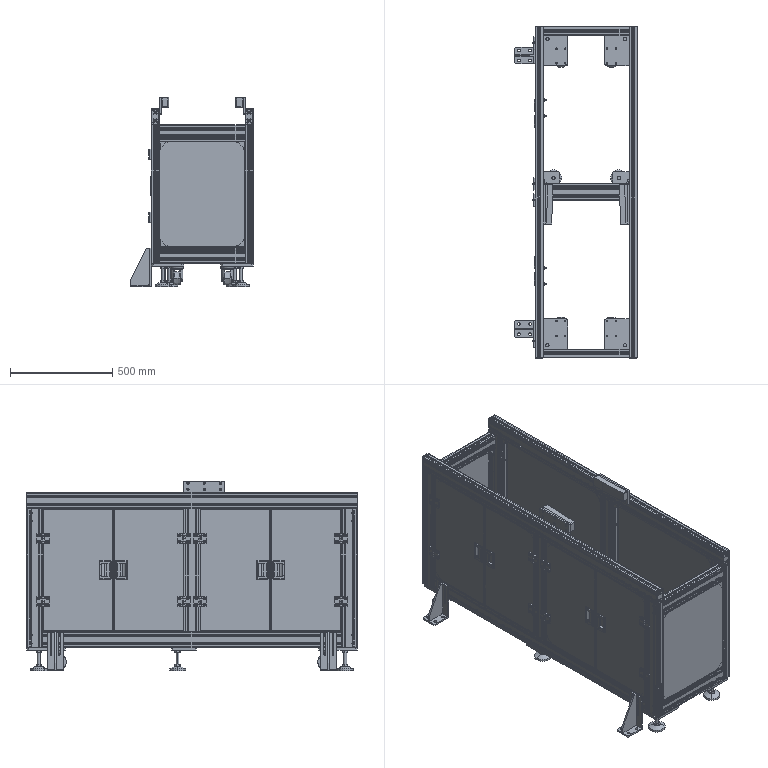Part | SolidWorks | 144 solids | 6684 faces | volume 27207263 mm3 | plane 4132 | cylinder 1976 | cone 460 | spline 104 | torus 12 | commonest cylinder face diameters 10 x236 9 x232 4 x208 8.5 x152 6.6 x132 8 x128